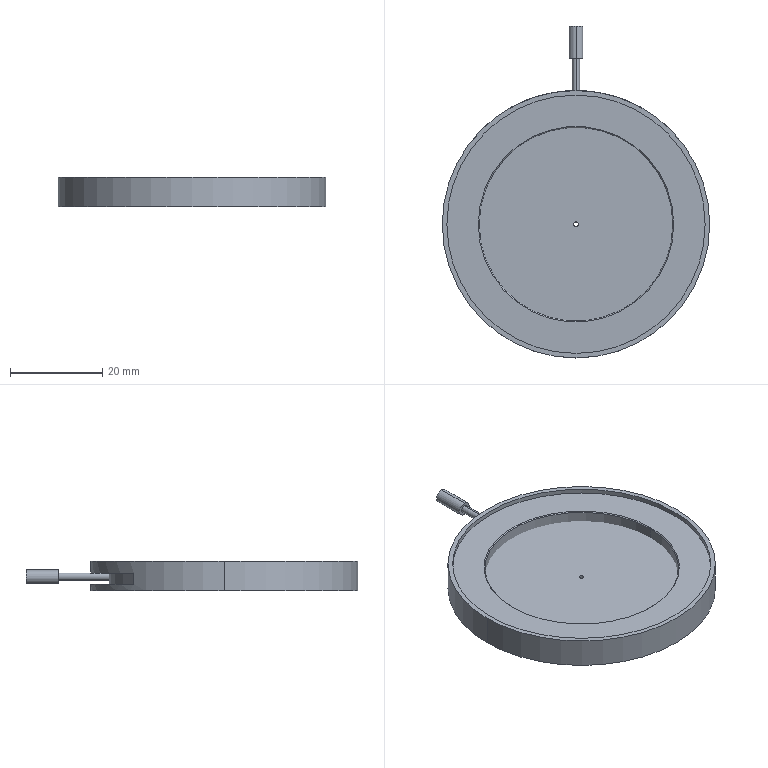Part | SolidWorks | features ICE 3, Chamfer 1, Extrusion 1, MoveFace 1, Revolution 1 | 3 solids | 29 faces | box 58 x 72 x 6.5 mm | volume 8321 mm3 | cylinder 15 | plane 12 | cone 2 | commonest cylinder face diameters 1 x2 1.6 x2 3 x2 42 x2 45 x2 56 x2
STEP:
#1=CARTESIAN_POINT('',(-21.,0.,5.3));
#2=VERTEX_POINT('',#1);
#3=CARTESIAN_POINT('',(21.,0.,5.3));
#4=VERTEX_POINT('',#3);
#5=CARTESIAN_POINT('',(0.,0.,5.3));
#6=DIRECTION('',(0.,0.,1.));
#7=DIRECTION('',(1.,0.,0.));
#8=AXIS2_PLACEMENT_3D('',#5,#6,#7);
#9=CIRCLE('',#8,21.);
#10=EDGE_CURVE('',#2,#4,#9,.T.);
#11=ORIENTED_EDGE('',*,*,#10,.F.);
#12=CARTESIAN_POINT('',(-21.2,0.,5.5));
#13=VERTEX_POINT('',#12);
#14=CARTESIAN_POINT('',(-21.,0.,5.3));
#15=DIRECTION('',(-0.7071,0.,0.7071));
#16=VECTOR('',#15,1000.);
#17=LINE('',#14,#16);
#18=EDGE_CURVE('',#2,#13,#17,.T.);
#19=ORIENTED_EDGE('',*,*,#18,.T.);
#20=CARTESIAN_POINT('',(21.2,0.,5.5));
#21=VERTEX_POINT('',#20);
#22=CARTESIAN_POINT('',(0.,0.,5.5));
#23=DIRECTION('',(0.,0.,-1.));
#24=DIRECTION('',(1.,0.,0.));
#25=AXIS2_PLACEMENT_3D('',#22,#23,#24);
#26=CIRCLE('',#25,21.2);
#27=EDGE_CURVE('',#21,#13,#26,.T.);
#28=ORIENTED_EDGE('',*,*,#27,.F.);
#29=CARTESIAN_POINT('',(21.,0.,5.3));
#30=DIRECTION('',(0.7071,0.,0.7071));
#31=VECTOR('',#30,1000.);
#32=LINE('',#29,#31);
#33=EDGE_CURVE('',#4,#21,#32,.T.);
#34=ORIENTED_EDGE('',*,*,#33,.F.);
#35=EDGE_LOOP('',(#11,#19,#28,#34));
#36=FACE_OUTER_BOUND('',#35,.T.);
#37=CARTESIAN_POINT('',(0.,0.,5.3));
#38=DIRECTION('',(0.,0.,1.));
#39=DIRECTION('',(1.,0.,0.));
#40=AXIS2_PLACEMENT_3D('',#37,#38,#39);
#41=CONICAL_SURFACE('',#40,21.,0.7854);
#42=ADVANCED_FACE('',(#36),#41,.F.);
#43=CARTESIAN_POINT('',(-28.,0.,5.5));
#44=VERTEX_POINT('',#43);
#45=CARTESIAN_POINT('',(28.,0.,5.5));
#46=VERTEX_POINT('',#45);
#47=CARTESIAN_POINT('',(0.,0.,5.5));
#48=DIRECTION('',(0.,0.,1.));
#49=DIRECTION('',(1.,0.,0.));
#50=AXIS2_PLACEMENT_3D('',#47,#48,#49);
#51=CIRCLE('',#50,28.);
#52=EDGE_CURVE('',#44,#46,#51,.T.);
#53=ORIENTED_EDGE('',*,*,#52,.F.);
#54=CARTESIAN_POINT('',(-28.,0.,6.5));
#55=VERTEX_POINT('',#54);
#56=CARTESIAN_POINT('',(-28.,0.,5.5));
#57=DIRECTION('',(0.,0.,1.));
#58=VECTOR('',#57,1000.);
#59=LINE('',#56,#58);
#60=EDGE_CURVE('',#44,#55,#59,.T.);
#61=ORIENTED_EDGE('',*,*,#60,.T.);
#62=CARTESIAN_POINT('',(28.,0.,6.5));
#63=VERTEX_POINT('',#62);
#64=CARTESIAN_POINT('',(0.,0.,6.5));
#65=DIRECTION('',(0.,0.,1.));
#66=DIRECTION('',(1.,0.,0.));
#67=AXIS2_PLACEMENT_3D('',#64,#65,#66);
#68=CIRCLE('',#67,28.);
#69=EDGE_CURVE('',#55,#63,#68,.T.);
#70=ORIENTED_EDGE('',*,*,#69,.T.);
#71=CARTESIAN_POINT('',(28.,0.,5.5));
#72=DIRECTION('',(0.,0.,1.));
#73=VECTOR('',#72,1000.);
#74=LINE('',#71,#73);
#75=EDGE_CURVE('',#46,#63,#74,.T.);
#76=ORIENTED_EDGE('',*,*,#75,.F.);
#77=EDGE_LOOP('',(#53,#61,#70,#76));
#78=FACE_OUTER_BOUND('',#77,.T.);
#79=CARTESIAN_POINT('',(0.,0.,5.5));
#80=DIRECTION('',(0.,0.,1.));
#81=DIRECTION('',(1.,0.,0.));
#82=AXIS2_PLACEMENT_3D('',#79,#80,#81);
#83=CYLINDRICAL_SURFACE('',#82,28.);
#84=ADVANCED_FACE('',(#78),#83,.F.);
#85=ORIENTED_EDGE('',*,*,#10,.T.);
#86=CARTESIAN_POINT('',(21.,0.,0.));
#87=VERTEX_POINT('',#86);
#88=CARTESIAN_POINT('',(21.,0.,6.5));
#89=DIRECTION('',(0.,0.,-1.));
#90=VECTOR('',#89,1000.);
#91=LINE('',#88,#90);
#92=EDGE_CURVE('',#4,#87,#91,.T.);
#93=ORIENTED_EDGE('',*,*,#92,.T.);
#94=CARTESIAN_POINT('',(-21.,0.,0.));
#95=VERTEX_POINT('',#94);
#96=CARTESIAN_POINT('',(0.,0.,0.));
#97=DIRECTION('',(0.,0.,1.));
#98=DIRECTION('',(1.,0.,0.));
#99=AXIS2_PLACEMENT_3D('',#96,#97,#98);
#100=CIRCLE('',#99,21.);
#101=EDGE_CURVE('',#95,#87,#100,.T.);
#102=ORIENTED_EDGE('',*,*,#101,.F.);
#103=CARTESIAN_POINT('',(-21.,0.,6.5));
#104=DIRECTION('',(0.,0.,-1.));
#105=VECTOR('',#104,1000.);
#106=LINE('',#103,#105);
#107=EDGE_CURVE('',#2,#95,#106,.T.);
#108=ORIENTED_EDGE('',*,*,#107,.F.);
#109=EDGE_LOOP('',(#85,#93,#102,#108));
#110=FACE_OUTER_BOUND('',#109,.T.);
#111=CARTESIAN_POINT('',(0.,0.,6.5));
#112=DIRECTION('',(0.,0.,-1.));
#113=DIRECTION('',(-1.,0.,0.));
#114=AXIS2_PLACEMENT_3D('',#111,#112,#113);
#115=CYLINDRICAL_SURFACE('',#114,21.);
#116=ADVANCED_FACE('',(#110),#115,.F.);
#117=CARTESIAN_POINT('',(-21.381,19.592,3.9));
#118=VERTEX_POINT('',#117);
#119=CARTESIAN_POINT('',(21.381,19.592,3.9));
#120=VERTEX_POINT('',#119);
#121=CARTESIAN_POINT('',(0.,0.,3.9));
#122=DIRECTION('',(0.,0.,-1.));
#123=DIRECTION('',(-1.,0.,0.));
#124=AXIS2_PLACEMENT_3D('',#121,#122,#123);
#125=CIRCLE('',#124,29.);
#126=EDGE_CURVE('',#118,#120,#125,.T.);
#127=ORIENTED_EDGE('',*,*,#126,.F.);
#128=CARTESIAN_POINT('',(-21.381,19.592,1.5));
#129=VERTEX_POINT('',#128);
#130=CARTESIAN_POINT('',(-21.381,19.592,3.9));
#131=DIRECTION('',(0.,0.,-1.));
#132=VECTOR('',#131,1000.);
#133=LINE('',#130,#132);
#134=EDGE_CURVE('',#118,#129,#133,.T.);
#135=ORIENTED_EDGE('',*,*,#134,.T.);
#136=CARTESIAN_POINT('',(21.381,19.592,1.5));
#137=VERTEX_POINT('',#136);
#138=CARTESIAN_POINT('',(0.,0.,1.5));
#139=DIRECTION('',(0.,0.,-1.));
#140=DIRECTION('',(-1.,0.,0.));
#141=AXIS2_PLACEMENT_3D('',#138,#139,#140);
#142=CIRCLE('',#141,29.);
#143=EDGE_CURVE('',#129,#137,#142,.T.);
#144=ORIENTED_EDGE('',*,*,#143,.T.);
#145=CARTESIAN_POINT('',(21.381,19.592,3.9));
#146=DIRECTION('',(0.,0.,-1.));
#147=VECTOR('',#146,1000.);
#148=LINE('',#145,#147);
#149=EDGE_CURVE('',#120,#137,#148,.T.);
#150=ORIENTED_EDGE('',*,*,#149,.F.);
#151=EDGE_LOOP('',(#127,#135,#144,#150));
#152=FACE_BOUND('',#151,.T.);
#153=CARTESIAN_POINT('',(29.,0.,6.5));
#154=VERTEX_POINT('',#153);
#155=CARTESIAN_POINT('',(-29.,0.,6.5));
#156=VERTEX_POINT('',#155);
#157=CARTESIAN_POINT('',(0.,0.,6.5));
#158=DIRECTION('',(0.,0.,1.));
#159=DIRECTION('',(1.,0.,0.));
#160=AXIS2_PLACEMENT_3D('',#157,#158,#159);
#161=CIRCLE('',#160,29.);
#162=EDGE_CURVE('',#154,#156,#161,.T.);
#163=ORIENTED_EDGE('',*,*,#162,.F.);
#164=CARTESIAN_POINT('',(29.,0.,0.));
#165=VERTEX_POINT('',#164);
#166=CARTESIAN_POINT('',(29.,0.,6.5));
#167=DIRECTION('',(0.,0.,-1.));
#168=VECTOR('',#167,1000.);
#169=LINE('',#166,#168);
#170=EDGE_CURVE('',#154,#165,#169,.T.);
#171=ORIENTED_EDGE('',*,*,#170,.T.);
#172=CARTESIAN_POINT('',(-29.,0.,0.));
#173=VERTEX_POINT('',#172);
#174=CARTESIAN_POINT('',(0.,0.,0.));
#175=DIRECTION('',(0.,0.,1.));
#176=DIRECTION('',(1.,0.,0.));
#177=AXIS2_PLACEMENT_3D('',#174,#175,#176);
#178=CIRCLE('',#177,29.);
#179=EDGE_CURVE('',#165,#173,#178,.T.);
#180=ORIENTED_EDGE('',*,*,#179,.T.);
#181=CARTESIAN_POINT('',(-29.,0.,6.5));
#182=DIRECTION('',(0.,0.,-1.));
#183=VECTOR('',#182,1000.);
#184=LINE('',#181,#183);
#185=EDGE_CURVE('',#156,#173,#184,.T.);
#186=ORIENTED_EDGE('',*,*,#185,.F.);
#187=EDGE_LOOP('',(#163,#171,#180,#186));
#188=FACE_OUTER_BOUND('',#187,.T.);
#189=CARTESIAN_POINT('',(0.,0.,6.5));
#190=DIRECTION('',(0.,0.,-1.));
#191=DIRECTION('',(-1.,0.,0.));
#192=AXIS2_PLACEMENT_3D('',#189,#190,#191);
#193=CYLINDRICAL_SURFACE('',#192,29.);
#194=ADVANCED_FACE('',(#152,#188),#193,.T.);
#195=ORIENTED_EDGE('',*,*,#170,.F.);
#196=CARTESIAN_POINT('',(0.,0.,6.5));
#197=DIRECTION('',(0.,0.,1.));
#198=DIRECTION('',(1.,0.,0.));
#199=AXIS2_PLACEMENT_3D('',#196,#197,#198);
#200=CIRCLE('',#199,29.);
#201=EDGE_CURVE('',#156,#154,#200,.T.);
#202=ORIENTED_EDGE('',*,*,#201,.F.);
#203=ORIENTED_EDGE('',*,*,#185,.T.);
#204=CARTESIAN_POINT('',(0.,0.,0.));
#205=DIRECTION('',(0.,0.,1.));
#206=DIRECTION('',(1.,0.,0.));
#207=AXIS2_PLACEMENT_3D('',#204,#205,#206);
#208=CIRCLE('',#207,29.);
#209=EDGE_CURVE('',#173,#165,#208,.T.);
#210=ORIENTED_EDGE('',*,*,#209,.T.);
#211=EDGE_LOOP('',(#195,#202,#203,#210));
#212=FACE_OUTER_BOUND('',#211,.T.);
#213=CARTESIAN_POINT('',(0.,0.,6.5));
#214=DIRECTION('',(0.,0.,-1.));
#215=DIRECTION('',(-1.,0.,0.));
#216=AXIS2_PLACEMENT_3D('',#213,#214,#215);
#217=CYLINDRICAL_SURFACE('',#216,29.);
#218=ADVANCED_FACE('',(#212),#217,.T.);
#219=ORIENTED_EDGE('',*,*,#92,.F.);
#220=CARTESIAN_POINT('',(0.,0.,5.3));
#221=DIRECTION('',(0.,0.,1.));
#222=DIRECTION('',(1.,0.,0.));
#223=AXIS2_PLACEMENT_3D('',#220,#221,#222);
#224=CIRCLE('',#223,21.);
#225=EDGE_CURVE('',#4,#2,#224,.T.);
#226=ORIENTED_EDGE('',*,*,#225,.T.);
#227=ORIENTED_EDGE('',*,*,#107,.T.);
#228=CARTESIAN_POINT('',(0.,0.,0.));
#229=DIRECTION('',(0.,0.,1.));
#230=DIRECTION('',(1.,0.,0.));
#231=AXIS2_PLACEMENT_3D('',#228,#229,#230);
#232=CIRCLE('',#231,21.);
#233=EDGE_CURVE('',#87,#95,#232,.T.);
#234=ORIENTED_EDGE('',*,*,#233,.F.);
#235=EDGE_LOOP('',(#219,#226,#227,#234));
#236=FACE_OUTER_BOUND('',#235,.T.);
#237=CARTESIAN_POINT('',(0.,0.,6.5));
#238=DIRECTION('',(0.,0.,-1.));
#239=DIRECTION('',(-1.,0.,0.));
#240=AXIS2_PLACEMENT_3D('',#237,#238,#239);
#241=CYLINDRICAL_SURFACE('',#240,21.);
#242=ADVANCED_FACE('',(#236),#241,.F.);
#243=CARTESIAN_POINT('',(0.,0.,6.5));
#244=DIRECTION('',(0.,0.,1.));
#245=DIRECTION('',(1.,0.,0.));
#246=AXIS2_PLACEMENT_3D('',#243,#244,#245);
#247=CIRCLE('',#246,28.);
#248=EDGE_CURVE('',#63,#55,#247,.T.);
#249=ORIENTED_EDGE('',*,*,#248,.F.);
#250=ORIENTED_EDGE('',*,*,#69,.F.);
#251=EDGE_LOOP('',(#249,#250));
#252=FACE_BOUND('',#251,.T.);
#253=ORIENTED_EDGE('',*,*,#201,.T.);
#254=ORIENTED_EDGE('',*,*,#162,.T.);
#255=EDGE_LOOP('',(#253,#254));
#256=FACE_OUTER_BOUND('',#255,.T.);
#257=CARTESIAN_POINT('',(0.,0.,6.5));
#258=DIRECTION('',(0.,0.,1.));
#259=DIRECTION('',(1.,0.,0.));
#260=AXIS2_PLACEMENT_3D('',#257,#258,#259);
#261=PLANE('',#260);
#262=ADVANCED_FACE('',(#252,#256),#261,.T.);
#263=ORIENTED_EDGE('',*,*,#209,.F.);
#264=ORIENTED_EDGE('',*,*,#179,.F.);
#265=EDGE_LOOP('',(#263,#264));
#266=FACE_OUTER_BOUND('',#265,.T.);
#267=ORIENTED_EDGE('',*,*,#101,.T.);
#268=ORIENTED_EDGE('',*,*,#233,.T.);
#269=EDGE_LOOP('',(#267,#268));
#270=FACE_BOUND('',#269,.T.);
#271=CARTESIAN_POINT('',(0.,0.,0.));
#272=DIRECTION('',(0.,0.,1.));
#273=DIRECTION('',(1.,0.,0.));
#274=AXIS2_PLACEMENT_3D('',#271,#272,#273);
#275=PLANE('',#274);
#276=ADVANCED_FACE('',(#266,#270),#275,.F.);
#277=ORIENTED_EDGE('',*,*,#60,.F.);
#278=CARTESIAN_POINT('',(0.,0.,5.5));
#279=DIRECTION('',(0.,0.,1.));
#280=DIRECTION('',(1.,0.,0.));
#281=AXIS2_PLACEMENT_3D('',#278,#279,#280);
#282=CIRCLE('',#281,28.);
#283=EDGE_CURVE('',#46,#44,#282,.T.);
#284=ORIENTED_EDGE('',*,*,#283,.F.);
#285=ORIENTED_EDGE('',*,*,#75,.T.);
#286=ORIENTED_EDGE('',*,*,#248,.T.);
#287=EDGE_LOOP('',(#277,#284,#285,#286));
#288=FACE_OUTER_BOUND('',#287,.T.);
#289=CARTESIAN_POINT('',(0.,0.,5.5));
#290=DIRECTION('',(0.,0.,1.));
#291=DIRECTION('',(1.,0.,0.));
#292=AXIS2_PLACEMENT_3D('',#289,#290,#291);
#293=CYLINDRICAL_SURFACE('',#292,28.);
#294=ADVANCED_FACE('',(#288),#293,.F.);
#295=ORIENTED_EDGE('',*,*,#27,.T.);
#296=CARTESIAN_POINT('',(0.,0.,5.5));
#297=DIRECTION('',(0.,0.,-1.));
#298=DIRECTION('',(1.,0.,0.));
#299=AXIS2_PLACEMENT_3D('',#296,#297,#298);
#300=CIRCLE('',#299,21.2);
#301=EDGE_CURVE('',#13,#21,#300,.T.);
#302=ORIENTED_EDGE('',*,*,#301,.T.);
#303=EDGE_LOOP('',(#295,#302));
#304=FACE_BOUND('',#303,.T.);
#305=ORIENTED_EDGE('',*,*,#283,.T.);
#306=ORIENTED_EDGE('',*,*,#52,.T.);
#307=EDGE_LOOP('',(#305,#306));
#308=FACE_OUTER_BOUND('',#307,.T.);
#309=CARTESIAN_POINT('',(0.,0.,5.5));
#310=DIRECTION('',(0.,0.,1.));
#311=DIRECTION('',(1.,0.,0.));
#312=AXIS2_PLACEMENT_3D('',#309,#310,#311);
#313=PLANE('',#312);
#314=ADVANCED_FACE('',(#304,#308),#313,.T.);
#315=CARTESIAN_POINT('',(-18.432,16.89,1.5));
#316=VERTEX_POINT('',#315);
#317=CARTESIAN_POINT('',(-18.432,16.89,1.5));
#318=DIRECTION('',(-0.7373,0.6756,0.));
#319=VECTOR('',#318,1000.);
#320=LINE('',#317,#319);
#321=EDGE_CURVE('',#316,#129,#320,.T.);
#322=ORIENTED_EDGE('',*,*,#321,.T.);
#323=ORIENTED_EDGE('',*,*,#134,.F.);
#324=CARTESIAN_POINT('',(-18.432,16.89,3.9));
#325=VERTEX_POINT('',#324);
#326=CARTESIAN_POINT('',(-18.432,16.89,3.9));
#327=DIRECTION('',(-0.7373,0.6756,0.));
#328=VECTOR('',#327,1000.);
#329=LINE('',#326,#328);
#330=EDGE_CURVE('',#325,#118,#329,.T.);
#331=ORIENTED_EDGE('',*,*,#330,.F.);
#332=CARTESIAN_POINT('',(-18.432,16.89,3.9));
#333=DIRECTION('',(0.,0.,-1.));
#334=VECTOR('',#333,1000.);
#335=LINE('',#332,#334);
#336=EDGE_CURVE('',#325,#316,#335,.T.);
#337=ORIENTED_EDGE('',*,*,#336,.T.);
#338=EDGE_LOOP('',(#322,#323,#331,#337));
#339=FACE_OUTER_BOUND('',#338,.T.);
#340=CARTESIAN_POINT('',(-18.432,16.89,3.9));
#341=DIRECTION('',(-0.6756,-0.7373,0.));
#342=DIRECTION('',(0.7373,-0.6756,0.));
#343=AXIS2_PLACEMENT_3D('',#340,#341,#342);
#344=PLANE('',#343);
#345=ADVANCED_FACE('',(#339),#344,.F.);
#346=CARTESIAN_POINT('',(18.432,16.89,1.5));
#347=VERTEX_POINT('',#346);
#348=CARTESIAN_POINT('',(0.,0.,1.5));
#349=DIRECTION('',(0.,0.,1.));
#350=DIRECTION('',(-1.,0.,0.));
#351=AXIS2_PLACEMENT_3D('',#348,#349,#350);
#352=CIRCLE('',#351,25.);
#353=EDGE_CURVE('',#347,#316,#352,.T.);
#354=ORIENTED_EDGE('',*,*,#353,.T.);
#355=ORIENTED_EDGE('',*,*,#336,.F.);
#356=CARTESIAN_POINT('',(18.432,16.89,3.9));
#357=VERTEX_POINT('',#356);
#358=CARTESIAN_POINT('',(0.,0.,3.9));
#359=DIRECTION('',(0.,0.,1.));
#360=DIRECTION('',(-1.,0.,0.));
#361=AXIS2_PLACEMENT_3D('',#358,#359,#360);
#362=CIRCLE('',#361,25.);
#363=EDGE_CURVE('',#357,#325,#362,.T.);
#364=ORIENTED_EDGE('',*,*,#363,.F.);
#365=CARTESIAN_POINT('',(18.432,16.89,3.9));
#366=DIRECTION('',(0.,0.,-1.));
#367=VECTOR('',#366,1000.);
#368=LINE('',#365,#367);
#369=EDGE_CURVE('',#357,#347,#368,.T.);
#370=ORIENTED_EDGE('',*,*,#369,.T.);
#371=EDGE_LOOP('',(#354,#355,#364,#370));
#372=FACE_OUTER_BOUND('',#371,.T.);
#373=CARTESIAN_POINT('',(0.,0.,3.9));
#374=DIRECTION('',(0.,0.,-1.));
#375=DIRECTION('',(-1.,0.,0.));
#376=AXIS2_PLACEMENT_3D('',#373,#374,#375);
#377=CYLINDRICAL_SURFACE('',#376,25.);
#378=ADVANCED_FACE('',(#372),#377,.T.);
#379=CARTESIAN_POINT('',(18.432,16.89,1.5));
#380=DIRECTION('',(-0.7373,-0.6756,0.));
#381=VECTOR('',#380,1000.);
#382=LINE('',#379,#381);
#383=EDGE_CURVE('',#137,#347,#382,.T.);
#384=ORIENTED_EDGE('',*,*,#383,.T.);
#385=ORIENTED_EDGE('',*,*,#369,.F.);
#386=CARTESIAN_POINT('',(18.432,16.89,3.9));
#387=DIRECTION('',(-0.7373,-0.6756,0.));
#388=VECTOR('',#387,1000.);
#389=LINE('',#386,#388);
#390=EDGE_CURVE('',#120,#357,#389,.T.);
#391=ORIENTED_EDGE('',*,*,#390,.F.);
#392=ORIENTED_EDGE('',*,*,#149,.T.);
#393=EDGE_LOOP('',(#384,#385,#391,#392));
#394=FACE_OUTER_BOUND('',#393,.T.);
#395=CARTESIAN_POINT('',(18.432,16.89,3.9));
#396=DIRECTION('',(0.6756,-0.7373,0.));
#397=DIRECTION('',(0.7373,0.6756,0.));
#398=AXIS2_PLACEMENT_3D('',#395,#396,#397);
#399=PLANE('',#398);
#400=ADVANCED_FACE('',(#394),#399,.F.);
#401=ORIENTED_EDGE('',*,*,#126,.T.);
#402=ORIENTED_EDGE('',*,*,#390,.T.);
#403=ORIENTED_EDGE('',*,*,#363,.T.);
#404=ORIENTED_EDGE('',*,*,#330,.T.);
#405=EDGE_LOOP('',(#401,#402,#403,#404));
#406=FACE_OUTER_BOUND('',#405,.T.);
#407=CARTESIAN_POINT('',(0.,0.,3.9));
#408=DIRECTION('',(0.,0.,-1.));
#409=DIRECTION('',(-1.,0.,0.));
#410=AXIS2_PLACEMENT_3D('',#407,#408,#409);
#411=PLANE('',#410);
#412=ADVANCED_FACE('',(#406),#411,.T.);
#413=ORIENTED_EDGE('',*,*,#143,.F.);
#414=ORIENTED_EDGE('',*,*,#321,.F.);
#415=ORIENTED_EDGE('',*,*,#353,.F.);
#416=ORIENTED_EDGE('',*,*,#383,.F.);
#417=EDGE_LOOP('',(#413,#414,#415,#416));
#418=FACE_OUTER_BOUND('',#417,.T.);
#419=CARTESIAN_POINT('',(0.,0.,1.5));
#420=DIRECTION('',(0.,0.,-1.));
#421=DIRECTION('',(-1.,0.,0.));
#422=AXIS2_PLACEMENT_3D('',#419,#420,#421);
#423=PLANE('',#422);
#424=ADVANCED_FACE('',(#418),#423,.F.);
#425=ORIENTED_EDGE('',*,*,#18,.F.);
#426=ORIENTED_EDGE('',*,*,#225,.F.);
#427=ORIENTED_EDGE('',*,*,#33,.T.);
#428=ORIENTED_EDGE('',*,*,#301,.F.);
#429=EDGE_LOOP('',(#425,#426,#427,#428));
#430=FACE_OUTER_BOUND('',#429,.T.);
#431=CARTESIAN_POINT('',(0.,0.,5.3));
#432=DIRECTION('',(0.,0.,1.));
#433=DIRECTION('',(1.,0.,0.));
#434=AXIS2_PLACEMENT_3D('',#431,#432,#433);
#435=CONICAL_SURFACE('',#434,21.,0.7854);
#436=ADVANCED_FACE('',(#430),#435,.F.);
#437=CLOSED_SHELL('',(#42,#84,#116,#194,#218,#242,#262,#276,#294,#314,#345,#378,#400,#412,#424,#436));
#438=MANIFOLD_SOLID_BREP('',#437);
#439=CARTESIAN_POINT('',(0.,36.,2.297));
#440=VERTEX_POINT('',#439);
#441=CARTESIAN_POINT('',(0.,36.,3.897));
#442=VERTEX_POINT('',#441);
#443=CARTESIAN_POINT('',(0.,36.,3.097));
#444=DIRECTION('',(0.,-1.,0.));
#445=DIRECTION('',(0.,0.,-1.));
#446=AXIS2_PLACEMENT_3D('',#443,#444,#445);
#447=CIRCLE('',#446,0.8);
#448=EDGE_CURVE('',#440,#442,#447,.T.);
#449=ORIENTED_EDGE('',*,*,#448,.T.);
#450=CARTESIAN_POINT('',(0.,24.,3.897));
#451=VERTEX_POINT('',#450);
#452=CARTESIAN_POINT('',(0.,29.,3.897));
#453=DIRECTION('',(0.,-1.,0.));
#454=VECTOR('',#453,1000.);
#455=LINE('',#452,#454);
#456=EDGE_CURVE('',#442,#451,#455,.T.);
#457=ORIENTED_EDGE('',*,*,#456,.T.);
#458=CARTESIAN_POINT('',(0.,24.,2.297));
#459=VERTEX_POINT('',#458);
#460=CARTESIAN_POINT('',(0.,24.,3.097));
#461=DIRECTION('',(0.,-1.,0.));
#462=DIRECTION('',(0.,0.,-1.));
#463=AXIS2_PLACEMENT_3D('',#460,#461,#462);
#464=CIRCLE('',#463,0.8);
#465=EDGE_CURVE('',#459,#451,#464,.T.);
#466=ORIENTED_EDGE('',*,*,#465,.F.);
#467=CARTESIAN_POINT('',(0.,29.,2.297));
#468=DIRECTION('',(0.,-1.,0.));
#469=VECTOR('',#468,1000.);
#470=LINE('',#467,#469);
#471=EDGE_CURVE('',#440,#459,#470,.T.);
#472=ORIENTED_EDGE('',*,*,#471,.F.);
#473=EDGE_LOOP('',(#449,#457,#466,#472));
#474=FACE_OUTER_BOUND('',#473,.T.);
#475=CARTESIAN_POINT('',(0.,29.,3.097));
#476=DIRECTION('',(0.,-1.,0.));
#477=DIRECTION('',(0.,0.,-1.));
#478=AXIS2_PLACEMENT_3D('',#475,#476,#477);
#479=CYLINDRICAL_SURFACE('',#478,0.8);
#480=ADVANCED_FACE('',(#474),#479,.T.);
#481=CARTESIAN_POINT('',(0.,43.,1.597));
#482=VERTEX_POINT('',#481);
#483=CARTESIAN_POINT('',(0.,43.,4.597));
#484=VERTEX_POINT('',#483);
#485=CARTESIAN_POINT('',(0.,43.,3.097));
#486=DIRECTION('',(0.,-1.,0.));
#487=DIRECTION('',(0.,0.,-1.));
#488=AXIS2_PLACEMENT_3D('',#485,#486,#487);
#489=CIRCLE('',#488,1.5);
#490=EDGE_CURVE('',#482,#484,#489,.T.);
#491=ORIENTED_EDGE('',*,*,#490,.T.);
#492=CARTESIAN_POINT('',(0.,36.,4.597));
#493=VERTEX_POINT('',#492);
#494=CARTESIAN_POINT('',(0.,29.,4.597));
#495=DIRECTION('',(0.,-1.,0.));
#496=VECTOR('',#495,1000.);
#497=LINE('',#494,#496);
#498=EDGE_CURVE('',#484,#493,#497,.T.);
#499=ORIENTED_EDGE('',*,*,#498,.T.);
#500=CARTESIAN_POINT('',(0.,36.,1.597));
#501=VERTEX_POINT('',#500);
#502=CARTESIAN_POINT('',(0.,36.,3.097));
#503=DIRECTION('',(0.,-1.,0.));
#504=DIRECTION('',(0.,0.,-1.));
#505=AXIS2_PLACEMENT_3D('',#502,#503,#504);
#506=CIRCLE('',#505,1.5);
#507=EDGE_CURVE('',#501,#493,#506,.T.);
#508=ORIENTED_EDGE('',*,*,#507,.F.);
#509=CARTESIAN_POINT('',(0.,29.,1.597));
#510=DIRECTION('',(0.,-1.,0.));
#511=VECTOR('',#510,1000.);
#512=LINE('',#509,#511);
#513=EDGE_CURVE('',#482,#501,#512,.T.);
#514=ORIENTED_EDGE('',*,*,#513,.F.);
#515=EDGE_LOOP('',(#491,#499,#508,#514));
#516=FACE_OUTER_BOUND('',#515,.T.);
#517=CARTESIAN_POINT('',(0.,29.,3.097));
#518=DIRECTION('',(0.,-1.,0.));
#519=DIRECTION('',(0.,0.,-1.));
#520=AXIS2_PLACEMENT_3D('',#517,#518,#519);
#521=CYLINDRICAL_SURFACE('',#520,1.5);
#522=ADVANCED_FACE('',(#516),#521,.T.);
#523=ORIENTED_EDGE('',*,*,#490,.F.);
#524=CARTESIAN_POINT('',(0.,43.,3.097));
#525=DIRECTION('',(0.,-1.,0.));
#526=DIRECTION('',(0.,0.,-1.));
#527=AXIS2_PLACEMENT_3D('',#524,#525,#526);
#528=CIRCLE('',#527,1.5);
#529=EDGE_CURVE('',#484,#482,#528,.T.);
#530=ORIENTED_EDGE('',*,*,#529,.F.);
#531=EDGE_LOOP('',(#523,#530));
#532=FACE_OUTER_BOUND('',#531,.T.);
#533=CARTESIAN_POINT('',(0.,43.,3.097));
#534=DIRECTION('',(0.,1.,0.));
#535=DIRECTION('',(0.,0.,1.));
#536=AXIS2_PLACEMENT_3D('',#533,#534,#535);
#537=PLANE('',#536);
#538=ADVANCED_FACE('',(#532),#537,.T.);
#539=ORIENTED_EDGE('',*,*,#498,.F.);
#540=ORIENTED_EDGE('',*,*,#529,.T.);
#541=ORIENTED_EDGE('',*,*,#513,.T.);
#542=CARTESIAN_POINT('',(0.,36.,3.097));
#543=DIRECTION('',(0.,-1.,0.));
#544=DIRECTION('',(0.,0.,-1.));
#545=AXIS2_PLACEMENT_3D('',#542,#543,#544);
#546=CIRCLE('',#545,1.5);
#547=EDGE_CURVE('',#493,#501,#546,.T.);
#548=ORIENTED_EDGE('',*,*,#547,.F.);
#549=EDGE_LOOP('',(#539,#540,#541,#548));
#550=FACE_OUTER_BOUND('',#549,.T.);
#551=CARTESIAN_POINT('',(0.,29.,3.097));
#552=DIRECTION('',(0.,-1.,0.));
#553=DIRECTION('',(0.,0.,-1.));
#554=AXIS2_PLACEMENT_3D('',#551,#552,#553);
#555=CYLINDRICAL_SURFACE('',#554,1.5);
#556=ADVANCED_FACE('',(#550),#555,.T.);
#557=ORIENTED_EDGE('',*,*,#507,.T.);
#558=ORIENTED_EDGE('',*,*,#547,.T.);
#559=EDGE_LOOP('',(#557,#558));
#560=FACE_OUTER_BOUND('',#559,.T.);
#561=ORIENTED_EDGE('',*,*,#448,.F.);
#562=CARTESIAN_POINT('',(0.,36.,3.097));
#563=DIRECTION('',(0.,-1.,0.));
#564=DIRECTION('',(0.,0.,-1.));
#565=AXIS2_PLACEMENT_3D('',#562,#563,#564);
#566=CIRCLE('',#565,0.8);
#567=EDGE_CURVE('',#442,#440,#566,.T.);
#568=ORIENTED_EDGE('',*,*,#567,.F.);
#569=EDGE_LOOP('',(#561,#568));
#570=FACE_BOUND('',#569,.T.);
#571=CARTESIAN_POINT('',(0.,36.,1.597));
#572=DIRECTION('',(0.,-1.,0.));
#573=DIRECTION('',(0.,0.,-1.));
#574=AXIS2_PLACEMENT_3D('',#571,#572,#573);
#575=PLANE('',#574);
#576=ADVANCED_FACE('',(#560,#570),#575,.T.);
#577=ORIENTED_EDGE('',*,*,#456,.F.);
#578=ORIENTED_EDGE('',*,*,#567,.T.);
#579=ORIENTED_EDGE('',*,*,#471,.T.);
#580=CARTESIAN_POINT('',(0.,24.,3.097));
#581=DIRECTION('',(0.,-1.,0.));
#582=DIRECTION('',(0.,0.,-1.));
#583=AXIS2_PLACEMENT_3D('',#580,#581,#582);
#584=CIRCLE('',#583,0.8);
#585=EDGE_CURVE('',#451,#459,#584,.T.);
#586=ORIENTED_EDGE('',*,*,#585,.F.);
#587=EDGE_LOOP('',(#577,#578,#579,#586));
#588=FACE_OUTER_BOUND('',#587,.T.);
#589=CARTESIAN_POINT('',(0.,29.,3.097));
#590=DIRECTION('',(0.,-1.,0.));
#591=DIRECTION('',(0.,0.,-1.));
#592=AXIS2_PLACEMENT_3D('',#589,#590,#591);
#593=CYLINDRICAL_SURFACE('',#592,0.8);
#594=ADVANCED_FACE('',(#588),#593,.T.);
#595=ORIENTED_EDGE('',*,*,#465,.T.);
#596=ORIENTED_EDGE('',*,*,#585,.T.);
#597=EDGE_LOOP('',(#595,#596));
#598=FACE_OUTER_BOUND('',#597,.T.);
#599=CARTESIAN_POINT('',(0.,24.,2.297));
#600=DIRECTION('',(0.,-1.,0.));
#601=DIRECTION('',(0.,0.,-1.));
#602=AXIS2_PLACEMENT_3D('',#599,#600,#601);
#603=PLANE('',#602);
#604=ADVANCED_FACE('',(#598),#603,.T.);
#605=CLOSED_SHELL('',(#480,#522,#538,#556,#576,#594,#604));
#606=MANIFOLD_SOLID_BREP('',#605);
#607=CARTESIAN_POINT('',(-0.5,0.,2.));
#608=VERTEX_POINT('',#607);
#609=CARTESIAN_POINT('',(0.5,0.,2.));
#610=VERTEX_POINT('',#609);
#611=CARTESIAN_POINT('',(0.,0.,2.));
#612=DIRECTION('',(0.,0.,1.));
#613=DIRECTION('',(1.,0.,0.));
#614=AXIS2_PLACEMENT_3D('',#611,#612,#613);
#615=CIRCLE('',#614,0.5);
#616=EDGE_CURVE('',#608,#610,#615,.T.);
#617=ORIENTED_EDGE('',*,*,#616,.F.);
#618=CARTESIAN_POINT('',(-0.5,0.,3.));
#619=VERTEX_POINT('',#618);
#620=CARTESIAN_POINT('',(-0.5,0.,2.));
#621=DIRECTION('',(0.,0.,1.));
#622=VECTOR('',#621,1000.);
#623=LINE('',#620,#622);
#624=EDGE_CURVE('',#608,#619,#623,.T.);
#625=ORIENTED_EDGE('',*,*,#624,.T.);
#626=CARTESIAN_POINT('',(0.5,0.,3.));
#627=VERTEX_POINT('',#626);
#628=CARTESIAN_POINT('',(0.,0.,3.));
#629=DIRECTION('',(0.,0.,1.));
#630=DIRECTION('',(1.,0.,0.));
#631=AXIS2_PLACEMENT_3D('',#628,#629,#630);
#632=CIRCLE('',#631,0.5);
#633=EDGE_CURVE('',#619,#627,#632,.T.);
#634=ORIENTED_EDGE('',*,*,#633,.T.);
#635=CARTESIAN_POINT('',(0.5,0.,2.));
#636=DIRECTION('',(0.,0.,1.));
#637=VECTOR('',#636,1000.);
#638=LINE('',#635,#637);
#639=EDGE_CURVE('',#610,#627,#638,.T.);
#640=ORIENTED_EDGE('',*,*,#639,.F.);
#641=EDGE_LOOP('',(#617,#625,#634,#640));
#642=FACE_OUTER_BOUND('',#641,.T.);
#643=CARTESIAN_POINT('',(0.,0.,2.));
#644=DIRECTION('',(0.,0.,1.));
#645=DIRECTION('',(1.,0.,0.));
#646=AXIS2_PLACEMENT_3D('',#643,#644,#645);
#647=CYLINDRICAL_SURFACE('',#646,0.5);
#648=ADVANCED_FACE('',(#642),#647,.F.);
#649=CARTESIAN_POINT('',(22.5,0.,2.));
#650=VERTEX_POINT('',#649);
#651=CARTESIAN_POINT('',(-22.5,0.,2.));
#652=VERTEX_POINT('',#651);
#653=CARTESIAN_POINT('',(0.,0.,2.));
#654=DIRECTION('',(0.,0.,1.));
#655=DIRECTION('',(1.,0.,0.));
#656=AXIS2_PLACEMENT_3D('',#653,#654,#655);
#657=CIRCLE('',#656,22.5);
#658=EDGE_CURVE('',#650,#652,#657,.T.);
#659=ORIENTED_EDGE('',*,*,#658,.T.);
#660=CARTESIAN_POINT('',(-22.5,0.,3.));
#661=VERTEX_POINT('',#660);
#662=CARTESIAN_POINT('',(-22.5,0.,2.));
#663=DIRECTION('',(0.,0.,1.));
#664=VECTOR('',#663,1000.);
#665=LINE('',#662,#664);
#666=EDGE_CURVE('',#652,#661,#665,.T.);
#667=ORIENTED_EDGE('',*,*,#666,.T.);
#668=CARTESIAN_POINT('',(22.5,0.,3.));
#669=VERTEX_POINT('',#668);
#670=CARTESIAN_POINT('',(0.,0.,3.));
#671=DIRECTION('',(0.,0.,1.));
#672=DIRECTION('',(1.,0.,0.));
#673=AXIS2_PLACEMENT_3D('',#670,#671,#672);
#674=CIRCLE('',#673,22.5);
#675=EDGE_CURVE('',#669,#661,#674,.T.);
#676=ORIENTED_EDGE('',*,*,#675,.F.);
#677=CARTESIAN_POINT('',(22.5,0.,2.));
#678=DIRECTION('',(0.,0.,1.));
#679=VECTOR('',#678,1000.);
#680=LINE('',#677,#679);
#681=EDGE_CURVE('',#650,#669,#680,.T.);
#682=ORIENTED_EDGE('',*,*,#681,.F.);
#683=EDGE_LOOP('',(#659,#667,#676,#682));
#684=FACE_OUTER_BOUND('',#683,.T.);
#685=CARTESIAN_POINT('',(0.,0.,2.));
#686=DIRECTION('',(0.,0.,1.));
#687=DIRECTION('',(1.,0.,0.));
#688=AXIS2_PLACEMENT_3D('',#685,#686,#687);
#689=CYLINDRICAL_SURFACE('',#688,22.5);
#690=ADVANCED_FACE('',(#684),#689,.T.);
#691=ORIENTED_EDGE('',*,*,#666,.F.);
#692=CARTESIAN_POINT('',(0.,0.,2.));
#693=DIRECTION('',(0.,0.,1.));
#694=DIRECTION('',(1.,0.,0.));
#695=AXIS2_PLACEMENT_3D('',#692,#693,#694);
#696=CIRCLE('',#695,22.5);
#697=EDGE_CURVE('',#652,#650,#696,.T.);
#698=ORIENTED_EDGE('',*,*,#697,.T.);
#699=ORIENTED_EDGE('',*,*,#681,.T.);
#700=CARTESIAN_POINT('',(0.,0.,3.));
#701=DIRECTION('',(0.,0.,1.));
#702=DIRECTION('',(1.,0.,0.));
#703=AXIS2_PLACEMENT_3D('',#700,#701,#702);
#704=CIRCLE('',#703,22.5);
#705=EDGE_CURVE('',#661,#669,#704,.T.);
#706=ORIENTED_EDGE('',*,*,#705,.F.);
#707=EDGE_LOOP('',(#691,#698,#699,#706));
#708=FACE_OUTER_BOUND('',#707,.T.);
#709=CARTESIAN_POINT('',(0.,0.,2.));
#710=DIRECTION('',(0.,0.,1.));
#711=DIRECTION('',(1.,0.,0.));
#712=AXIS2_PLACEMENT_3D('',#709,#710,#711);
#713=CYLINDRICAL_SURFACE('',#712,22.5);
#714=ADVANCED_FACE('',(#708),#713,.T.);
#715=CARTESIAN_POINT('',(0.,0.,2.));
#716=DIRECTION('',(0.,0.,1.));
#717=DIRECTION('',(1.,0.,0.));
#718=AXIS2_PLACEMENT_3D('',#715,#716,#717);
#719=CIRCLE('',#718,0.5);
#720=EDGE_CURVE('',#610,#608,#719,.T.);
#721=ORIENTED_EDGE('',*,*,#720,.T.);
#722=ORIENTED_EDGE('',*,*,#616,.T.);
#723=EDGE_LOOP('',(#721,#722));
#724=FACE_BOUND('',#723,.T.);
#725=ORIENTED_EDGE('',*,*,#658,.F.);
#726=ORIENTED_EDGE('',*,*,#697,.F.);
#727=EDGE_LOOP('',(#725,#726));
#728=FACE_OUTER_BOUND('',#727,.T.);
#729=CARTESIAN_POINT('',(0.,0.,2.));
#730=DIRECTION('',(0.,0.,1.));
#731=DIRECTION('',(1.,0.,0.));
#732=AXIS2_PLACEMENT_3D('',#729,#730,#731);
#733=PLANE('',#732);
#734=ADVANCED_FACE('',(#724,#728),#733,.F.);
#735=CARTESIAN_POINT('',(0.,0.,3.));
#736=DIRECTION('',(0.,0.,1.));
#737=DIRECTION('',(1.,0.,0.));
#738=AXIS2_PLACEMENT_3D('',#735,#736,#737);
#739=CIRCLE('',#738,0.5);
#740=EDGE_CURVE('',#627,#619,#739,.T.);
#741=ORIENTED_EDGE('',*,*,#740,.F.);
#742=ORIENTED_EDGE('',*,*,#633,.F.);
#743=EDGE_LOOP('',(#741,#742));
#744=FACE_BOUND('',#743,.T.);
#745=ORIENTED_EDGE('',*,*,#675,.T.);
#746=ORIENTED_EDGE('',*,*,#705,.T.);
#747=EDGE_LOOP('',(#745,#746));
#748=FACE_OUTER_BOUND('',#747,.T.);
#749=CARTESIAN_POINT('',(0.,0.,3.));
#750=DIRECTION('',(0.,0.,1.));
#751=DIRECTION('',(1.,0.,0.));
#752=AXIS2_PLACEMENT_3D('',#749,#750,#751);
#753=PLANE('',#752);
#754=ADVANCED_FACE('',(#744,#748),#753,.T.);
#755=ORIENTED_EDGE('',*,*,#624,.F.);
#756=ORIENTED_EDGE('',*,*,#720,.F.);
#757=ORIENTED_EDGE('',*,*,#639,.T.);
#758=ORIENTED_EDGE('',*,*,#740,.T.);
#759=EDGE_LOOP('',(#755,#756,#757,#758));
#760=FACE_OUTER_BOUND('',#759,.T.);
#761=CARTESIAN_POINT('',(0.,0.,2.));
#762=DIRECTION('',(0.,0.,1.));
#763=DIRECTION('',(1.,0.,0.));
#764=AXIS2_PLACEMENT_3D('',#761,#762,#763);
#765=CYLINDRICAL_SURFACE('',#764,0.5);
#766=ADVANCED_FACE('',(#760),#765,.F.);
#767=CLOSED_SHELL('',(#648,#690,#714,#734,#754,#766));
#768=MANIFOLD_SOLID_BREP('',#767);
#769=CARTESIAN_POINT('',(0.,0.,0.));
#770=DIRECTION('',(0.,0.,1.));
#771=DIRECTION('',(1.,0.,0.));
#772=AXIS2_PLACEMENT_3D('',#769,#770,#771);
#773=(LENGTH_UNIT()NAMED_UNIT(*)SI_UNIT(.MILLI.,.METRE.));
#774=UNCERTAINTY_MEASURE_WITH_UNIT(LENGTH_MEASURE(0.00001),#773,'','');
#775=(NAMED_UNIT(*)PLANE_ANGLE_UNIT()SI_UNIT($,.RADIAN.));
#776=(NAMED_UNIT(*)SI_UNIT($,.STERADIAN.)SOLID_ANGLE_UNIT());
#777=(GEOMETRIC_REPRESENTATION_CONTEXT(3)GLOBAL_UNCERTAINTY_ASSIGNED_CONTEXT((#774))GLOBAL_UNIT_ASSIGNED_CONTEXT((#773,#775,#776))REPRESENTATION_CONTEXT('',''));
#778=ADVANCED_BREP_SHAPE_REPRESENTATION('',(#438,#606,#768,#772),#777);